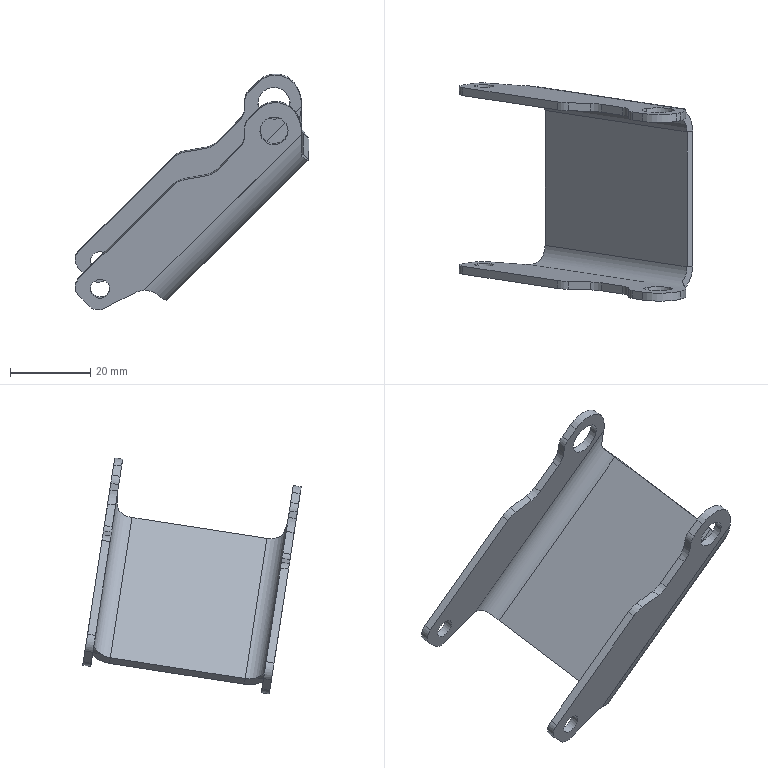Part | SolidWorks | features BaseBody 1 | 1 solid | 61 faces | box 58.154 x 54.417 x 58.795 mm | volume 8084 mm3 | cylinder 33 | plane 26 | spline 2 | commonest cylinder face diameters 10 x8 6 x6 4.8 x4 9 x3 12 x3 13 x3